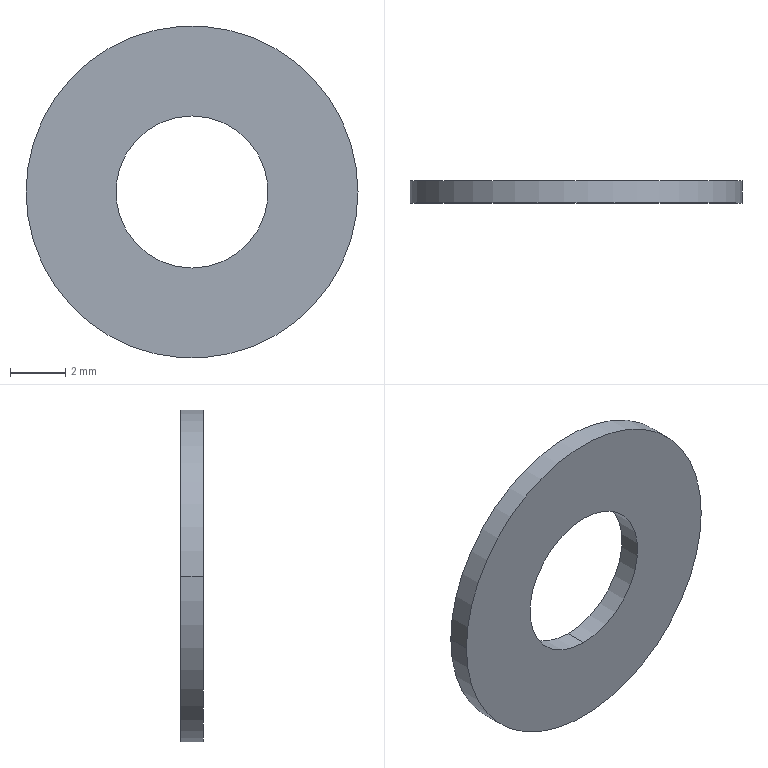Part | STEP file | ZZ21-M5 | 1 solid | 6 faces | box 12 x 0.8 x 12 mm | volume 71.471 mm3 | cylinder 4 | plane 2 | commonest cylinder face diameters 5.5 x2 12 x2
STEP:
#1=CARTESIAN_POINT('',(0.,0.,0.));
#2=DIRECTION('',(0.,0.,1.));
#3=DIRECTION('',(1.,0.,0.));
#4=AXIS2_PLACEMENT_3D('',#1,#2,#3);
#5=CARTESIAN_POINT('',(0.,0.,-2.75));
#6=VERTEX_POINT('',#5);
#7=CARTESIAN_POINT('',(0.,0.8,-2.75));
#8=VERTEX_POINT('',#7);
#9=CARTESIAN_POINT('',(0.,0.,-2.75));
#10=DIRECTION('',(0.,1.,0.));
#11=VECTOR('',#10,1.);
#12=LINE('',#9,#11);
#13=CARTESIAN_POINT('',(0.,0.,0.));
#14=DIRECTION('',(0.,1.,0.));
#15=DIRECTION('',(0.,0.,-1.));
#16=AXIS2_PLACEMENT_3D('',#13,#14,#15);
#17=CYLINDRICAL_SURFACE('',#16,2.75);
#18=CARTESIAN_POINT('',(6.283,0.));
#19=DIRECTION('',(0.,1.));
#20=VECTOR('',#19,1.);
#21=LINE('',#18,#20);
#22=(GEOMETRIC_REPRESENTATION_CONTEXT(2)PARAMETRIC_REPRESENTATION_CONTEXT()REPRESENTATION_CONTEXT('',''));
#23=DEFINITIONAL_REPRESENTATION('',(#21),#22);
#24=PCURVE('',#17,#23);
#25=CARTESIAN_POINT('',(0.,0.,0.));
#26=DIRECTION('',(0.,1.,0.));
#27=DIRECTION('',(0.,0.,-1.));
#28=AXIS2_PLACEMENT_3D('',#25,#26,#27);
#29=CYLINDRICAL_SURFACE('',#28,2.75);
#30=CARTESIAN_POINT('',(0.,0.));
#31=DIRECTION('',(0.,1.));
#32=VECTOR('',#31,1.);
#33=LINE('',#30,#32);
#34=(GEOMETRIC_REPRESENTATION_CONTEXT(2)PARAMETRIC_REPRESENTATION_CONTEXT()REPRESENTATION_CONTEXT('',''));
#35=DEFINITIONAL_REPRESENTATION('',(#33),#34);
#36=PCURVE('',#29,#35);
#37=SURFACE_CURVE('',#12,(#24,#36),.PCURVE_S1.);
#38=EDGE_CURVE('',#6,#8,#37,.T.);
#39=ORIENTED_EDGE('',*,*,#38,.T.);
#40=CARTESIAN_POINT('',(0.,0.8,2.75));
#41=VERTEX_POINT('',#40);
#42=CARTESIAN_POINT('',(0.,0.8,0.));
#43=DIRECTION('',(0.,-1.,0.));
#44=DIRECTION('',(0.,0.,1.));
#45=AXIS2_PLACEMENT_3D('',#42,#43,#44);
#46=CIRCLE('',#45,2.75);
#47=CARTESIAN_POINT('',(9.425,0.8));
#48=DIRECTION('',(-1.,0.));
#49=VECTOR('',#48,1.);
#50=LINE('',#47,#49);
#51=(GEOMETRIC_REPRESENTATION_CONTEXT(2)PARAMETRIC_REPRESENTATION_CONTEXT()REPRESENTATION_CONTEXT('',''));
#52=DEFINITIONAL_REPRESENTATION('',(#50),#51);
#53=PCURVE('',#17,#52);
#54=CARTESIAN_POINT('',(0.,0.8,0.));
#55=DIRECTION('',(0.,1.,0.));
#56=DIRECTION('',(-1.,0.,0.));
#57=AXIS2_PLACEMENT_3D('',#54,#55,#56);
#58=PLANE('',#57);
#59=CARTESIAN_POINT('',(0.,2.75));
#60=CARTESIAN_POINT('',(4.763,2.75));
#61=CARTESIAN_POINT('',(2.382,-1.375));
#62=CARTESIAN_POINT('',(0.,-5.5));
#63=CARTESIAN_POINT('',(-2.382,-1.375));
#64=CARTESIAN_POINT('',(-4.763,2.75));
#65=CARTESIAN_POINT('',(0.,2.75));
#66=(BOUNDED_CURVE()B_SPLINE_CURVE(2,(#59,#60,#61,#62,#63,#64,#65),.UNSPECIFIED.,.T.,.F.)B_SPLINE_CURVE_WITH_KNOTS((1,2,2,2,2,1),(-2.094,0.,2.094,4.189,6.283,8.378),.UNSPECIFIED.)CURVE()GEOMETRIC_REPRESENTATION_ITEM()RATIONAL_B_SPLINE_CURVE((1.,0.5,1.,0.5,1.,0.5,1.))REPRESENTATION_ITEM(''));
#67=(GEOMETRIC_REPRESENTATION_CONTEXT(2)PARAMETRIC_REPRESENTATION_CONTEXT()REPRESENTATION_CONTEXT('',''));
#68=DEFINITIONAL_REPRESENTATION('',(#66),#67);
#69=PCURVE('',#58,#68);
#70=SURFACE_CURVE('',#46,(#53,#69),.PCURVE_S1.);
#71=EDGE_CURVE('',#8,#41,#70,.T.);
#72=ORIENTED_EDGE('',*,*,#71,.T.);
#73=CARTESIAN_POINT('',(0.,0.,2.75));
#74=VERTEX_POINT('',#73);
#75=CARTESIAN_POINT('',(0.,0.,2.75));
#76=DIRECTION('',(0.,1.,0.));
#77=VECTOR('',#76,1.);
#78=LINE('',#75,#77);
#79=CARTESIAN_POINT('',(3.142,0.));
#80=DIRECTION('',(0.,1.));
#81=VECTOR('',#80,1.);
#82=LINE('',#79,#81);
#83=(GEOMETRIC_REPRESENTATION_CONTEXT(2)PARAMETRIC_REPRESENTATION_CONTEXT()REPRESENTATION_CONTEXT('',''));
#84=DEFINITIONAL_REPRESENTATION('',(#82),#83);
#85=PCURVE('',#17,#84);
#86=CARTESIAN_POINT('',(3.142,0.));
#87=DIRECTION('',(0.,1.));
#88=VECTOR('',#87,1.);
#89=LINE('',#86,#88);
#90=(GEOMETRIC_REPRESENTATION_CONTEXT(2)PARAMETRIC_REPRESENTATION_CONTEXT()REPRESENTATION_CONTEXT('',''));
#91=DEFINITIONAL_REPRESENTATION('',(#89),#90);
#92=PCURVE('',#29,#91);
#93=SURFACE_CURVE('',#78,(#85,#92),.PCURVE_S1.);
#94=EDGE_CURVE('',#74,#41,#93,.T.);
#95=ORIENTED_EDGE('',*,*,#94,.F.);
#96=CARTESIAN_POINT('',(0.,0.,0.));
#97=DIRECTION('',(0.,1.,0.));
#98=DIRECTION('',(0.,0.,-1.));
#99=AXIS2_PLACEMENT_3D('',#96,#97,#98);
#100=CIRCLE('',#99,2.75);
#101=CARTESIAN_POINT('',(0.,0.));
#102=DIRECTION('',(1.,0.));
#103=VECTOR('',#102,1.);
#104=LINE('',#101,#103);
#105=(GEOMETRIC_REPRESENTATION_CONTEXT(2)PARAMETRIC_REPRESENTATION_CONTEXT()REPRESENTATION_CONTEXT('',''));
#106=DEFINITIONAL_REPRESENTATION('',(#104),#105);
#107=PCURVE('',#17,#106);
#108=CARTESIAN_POINT('',(0.,0.,0.));
#109=DIRECTION('',(0.,-1.,0.));
#110=DIRECTION('',(1.,0.,0.));
#111=AXIS2_PLACEMENT_3D('',#108,#109,#110);
#112=PLANE('',#111);
#113=CARTESIAN_POINT('',(0.,-2.75));
#114=CARTESIAN_POINT('',(-4.763,-2.75));
#115=CARTESIAN_POINT('',(-2.382,1.375));
#116=CARTESIAN_POINT('',(0.,5.5));
#117=CARTESIAN_POINT('',(2.382,1.375));
#118=CARTESIAN_POINT('',(4.763,-2.75));
#119=CARTESIAN_POINT('',(0.,-2.75));
#120=(BOUNDED_CURVE()B_SPLINE_CURVE(2,(#113,#114,#115,#116,#117,#118,#119),.UNSPECIFIED.,.T.,.F.)B_SPLINE_CURVE_WITH_KNOTS((1,2,2,2,2,1),(-2.094,0.,2.094,4.189,6.283,8.378),.UNSPECIFIED.)CURVE()GEOMETRIC_REPRESENTATION_ITEM()RATIONAL_B_SPLINE_CURVE((1.,0.5,1.,0.5,1.,0.5,1.))REPRESENTATION_ITEM(''));
#121=(GEOMETRIC_REPRESENTATION_CONTEXT(2)PARAMETRIC_REPRESENTATION_CONTEXT()REPRESENTATION_CONTEXT('',''));
#122=DEFINITIONAL_REPRESENTATION('',(#120),#121);
#123=PCURVE('',#112,#122);
#124=SURFACE_CURVE('',#100,(#107,#123),.PCURVE_S1.);
#125=EDGE_CURVE('',#74,#6,#124,.T.);
#126=ORIENTED_EDGE('',*,*,#125,.T.);
#127=EDGE_LOOP('',(#39,#72,#95,#126));
#128=FACE_BOUND('',#127,.F.);
#129=ADVANCED_FACE('',(#128),#17,.F.);
#130=CARTESIAN_POINT('',(-6.,0.,0.));
#131=VERTEX_POINT('',#130);
#132=CARTESIAN_POINT('',(6.,0.,0.));
#133=VERTEX_POINT('',#132);
#134=CARTESIAN_POINT('',(0.,0.,0.));
#135=DIRECTION('',(0.,1.,0.));
#136=DIRECTION('',(-1.,0.,0.));
#137=AXIS2_PLACEMENT_3D('',#134,#135,#136);
#138=CIRCLE('',#137,6.);
#139=CARTESIAN_POINT('',(0.,0.,0.));
#140=DIRECTION('',(0.,1.,0.));
#141=DIRECTION('',(-1.,0.,0.));
#142=AXIS2_PLACEMENT_3D('',#139,#140,#141);
#143=CYLINDRICAL_SURFACE('',#142,6.);
#144=CARTESIAN_POINT('',(0.,0.));
#145=DIRECTION('',(1.,0.));
#146=VECTOR('',#145,1.);
#147=LINE('',#144,#146);
#148=(GEOMETRIC_REPRESENTATION_CONTEXT(2)PARAMETRIC_REPRESENTATION_CONTEXT()REPRESENTATION_CONTEXT('',''));
#149=DEFINITIONAL_REPRESENTATION('',(#147),#148);
#150=PCURVE('',#143,#149);
#151=CARTESIAN_POINT('',(-6.,0.));
#152=CARTESIAN_POINT('',(-6.,10.392));
#153=CARTESIAN_POINT('',(3.,5.196));
#154=CARTESIAN_POINT('',(12.,0.));
#155=CARTESIAN_POINT('',(3.,-5.196));
#156=CARTESIAN_POINT('',(-6.,-10.392));
#157=CARTESIAN_POINT('',(-6.,0.));
#158=(BOUNDED_CURVE()B_SPLINE_CURVE(2,(#151,#152,#153,#154,#155,#156,#157),.UNSPECIFIED.,.T.,.F.)B_SPLINE_CURVE_WITH_KNOTS((1,2,2,2,2,1),(-2.094,0.,2.094,4.189,6.283,8.378),.UNSPECIFIED.)CURVE()GEOMETRIC_REPRESENTATION_ITEM()RATIONAL_B_SPLINE_CURVE((1.,0.5,1.,0.5,1.,0.5,1.))REPRESENTATION_ITEM(''));
#159=(GEOMETRIC_REPRESENTATION_CONTEXT(2)PARAMETRIC_REPRESENTATION_CONTEXT()REPRESENTATION_CONTEXT('',''));
#160=DEFINITIONAL_REPRESENTATION('',(#158),#159);
#161=PCURVE('',#112,#160);
#162=SURFACE_CURVE('',#138,(#150,#161),.PCURVE_S1.);
#163=EDGE_CURVE('',#131,#133,#162,.T.);
#164=ORIENTED_EDGE('',*,*,#163,.T.);
#165=CARTESIAN_POINT('',(6.,0.8,0.));
#166=VERTEX_POINT('',#165);
#167=CARTESIAN_POINT('',(6.,0.,0.));
#168=DIRECTION('',(0.,1.,0.));
#169=VECTOR('',#168,1.);
#170=LINE('',#167,#169);
#171=CARTESIAN_POINT('',(3.142,0.));
#172=DIRECTION('',(0.,1.));
#173=VECTOR('',#172,1.);
#174=LINE('',#171,#173);
#175=(GEOMETRIC_REPRESENTATION_CONTEXT(2)PARAMETRIC_REPRESENTATION_CONTEXT()REPRESENTATION_CONTEXT('',''));
#176=DEFINITIONAL_REPRESENTATION('',(#174),#175);
#177=PCURVE('',#143,#176);
#178=CARTESIAN_POINT('',(0.,0.,0.));
#179=DIRECTION('',(0.,1.,0.));
#180=DIRECTION('',(-1.,0.,0.));
#181=AXIS2_PLACEMENT_3D('',#178,#179,#180);
#182=CYLINDRICAL_SURFACE('',#181,6.);
#183=CARTESIAN_POINT('',(3.142,0.));
#184=DIRECTION('',(0.,1.));
#185=VECTOR('',#184,1.);
#186=LINE('',#183,#185);
#187=(GEOMETRIC_REPRESENTATION_CONTEXT(2)PARAMETRIC_REPRESENTATION_CONTEXT()REPRESENTATION_CONTEXT('',''));
#188=DEFINITIONAL_REPRESENTATION('',(#186),#187);
#189=PCURVE('',#182,#188);
#190=SURFACE_CURVE('',#170,(#177,#189),.PCURVE_S1.);
#191=EDGE_CURVE('',#133,#166,#190,.T.);
#192=ORIENTED_EDGE('',*,*,#191,.T.);
#193=CARTESIAN_POINT('',(-6.,0.8,0.));
#194=VERTEX_POINT('',#193);
#195=CARTESIAN_POINT('',(0.,0.8,0.));
#196=DIRECTION('',(0.,-1.,0.));
#197=DIRECTION('',(1.,0.,0.));
#198=AXIS2_PLACEMENT_3D('',#195,#196,#197);
#199=CIRCLE('',#198,6.);
#200=CARTESIAN_POINT('',(3.142,0.8));
#201=DIRECTION('',(-1.,0.));
#202=VECTOR('',#201,1.);
#203=LINE('',#200,#202);
#204=(GEOMETRIC_REPRESENTATION_CONTEXT(2)PARAMETRIC_REPRESENTATION_CONTEXT()REPRESENTATION_CONTEXT('',''));
#205=DEFINITIONAL_REPRESENTATION('',(#203),#204);
#206=PCURVE('',#143,#205);
#207=CARTESIAN_POINT('',(-6.,0.));
#208=CARTESIAN_POINT('',(-6.,10.392));
#209=CARTESIAN_POINT('',(3.,5.196));
#210=CARTESIAN_POINT('',(12.,0.));
#211=CARTESIAN_POINT('',(3.,-5.196));
#212=CARTESIAN_POINT('',(-6.,-10.392));
#213=CARTESIAN_POINT('',(-6.,0.));
#214=(BOUNDED_CURVE()B_SPLINE_CURVE(2,(#207,#208,#209,#210,#211,#212,#213),.UNSPECIFIED.,.T.,.F.)B_SPLINE_CURVE_WITH_KNOTS((1,2,2,2,2,1),(-2.094,0.,2.094,4.189,6.283,8.378),.UNSPECIFIED.)CURVE()GEOMETRIC_REPRESENTATION_ITEM()RATIONAL_B_SPLINE_CURVE((1.,0.5,1.,0.5,1.,0.5,1.))REPRESENTATION_ITEM(''));
#215=(GEOMETRIC_REPRESENTATION_CONTEXT(2)PARAMETRIC_REPRESENTATION_CONTEXT()REPRESENTATION_CONTEXT('',''));
#216=DEFINITIONAL_REPRESENTATION('',(#214),#215);
#217=PCURVE('',#58,#216);
#218=SURFACE_CURVE('',#199,(#206,#217),.PCURVE_S1.);
#219=EDGE_CURVE('',#166,#194,#218,.T.);
#220=ORIENTED_EDGE('',*,*,#219,.T.);
#221=CARTESIAN_POINT('',(-6.,0.,0.));
#222=DIRECTION('',(0.,1.,0.));
#223=VECTOR('',#222,1.);
#224=LINE('',#221,#223);
#225=CARTESIAN_POINT('',(0.,0.));
#226=DIRECTION('',(0.,1.));
#227=VECTOR('',#226,1.);
#228=LINE('',#225,#227);
#229=(GEOMETRIC_REPRESENTATION_CONTEXT(2)PARAMETRIC_REPRESENTATION_CONTEXT()REPRESENTATION_CONTEXT('',''));
#230=DEFINITIONAL_REPRESENTATION('',(#228),#229);
#231=PCURVE('',#143,#230);
#232=CARTESIAN_POINT('',(6.283,0.));
#233=DIRECTION('',(0.,1.));
#234=VECTOR('',#233,1.);
#235=LINE('',#232,#234);
#236=(GEOMETRIC_REPRESENTATION_CONTEXT(2)PARAMETRIC_REPRESENTATION_CONTEXT()REPRESENTATION_CONTEXT('',''));
#237=DEFINITIONAL_REPRESENTATION('',(#235),#236);
#238=PCURVE('',#182,#237);
#239=SURFACE_CURVE('',#224,(#231,#238),.PCURVE_S1.);
#240=EDGE_CURVE('',#131,#194,#239,.T.);
#241=ORIENTED_EDGE('',*,*,#240,.F.);
#242=EDGE_LOOP('',(#164,#192,#220,#241));
#243=FACE_BOUND('',#242,.T.);
#244=ADVANCED_FACE('',(#243),#143,.T.);
#245=ORIENTED_EDGE('',*,*,#71,.T.);
#246=CARTESIAN_POINT('',(0.,0.8,0.));
#247=DIRECTION('',(0.,-1.,0.));
#248=DIRECTION('',(0.,0.,1.));
#249=AXIS2_PLACEMENT_3D('',#246,#247,#248);
#250=CIRCLE('',#249,2.75);
#251=CARTESIAN_POINT('',(0.,2.75));
#252=CARTESIAN_POINT('',(4.763,2.75));
#253=CARTESIAN_POINT('',(2.382,-1.375));
#254=CARTESIAN_POINT('',(0.,-5.5));
#255=CARTESIAN_POINT('',(-2.382,-1.375));
#256=CARTESIAN_POINT('',(-4.763,2.75));
#257=CARTESIAN_POINT('',(0.,2.75));
#258=(BOUNDED_CURVE()B_SPLINE_CURVE(2,(#251,#252,#253,#254,#255,#256,#257),.UNSPECIFIED.,.T.,.F.)B_SPLINE_CURVE_WITH_KNOTS((1,2,2,2,2,1),(-2.094,0.,2.094,4.189,6.283,8.378),.UNSPECIFIED.)CURVE()GEOMETRIC_REPRESENTATION_ITEM()RATIONAL_B_SPLINE_CURVE((1.,0.5,1.,0.5,1.,0.5,1.))REPRESENTATION_ITEM(''));
#259=(GEOMETRIC_REPRESENTATION_CONTEXT(2)PARAMETRIC_REPRESENTATION_CONTEXT()REPRESENTATION_CONTEXT('',''));
#260=DEFINITIONAL_REPRESENTATION('',(#258),#259);
#261=PCURVE('',#58,#260);
#262=CARTESIAN_POINT('',(3.142,0.8));
#263=DIRECTION('',(-1.,0.));
#264=VECTOR('',#263,1.);
#265=LINE('',#262,#264);
#266=(GEOMETRIC_REPRESENTATION_CONTEXT(2)PARAMETRIC_REPRESENTATION_CONTEXT()REPRESENTATION_CONTEXT('',''));
#267=DEFINITIONAL_REPRESENTATION('',(#265),#266);
#268=PCURVE('',#29,#267);
#269=SURFACE_CURVE('',#250,(#261,#268),.PCURVE_S1.);
#270=EDGE_CURVE('',#41,#8,#269,.T.);
#271=ORIENTED_EDGE('',*,*,#270,.T.);
#272=EDGE_LOOP('',(#245,#271));
#273=FACE_BOUND('',#272,.T.);
#274=CARTESIAN_POINT('',(0.,0.8,0.));
#275=DIRECTION('',(0.,-1.,0.));
#276=DIRECTION('',(1.,0.,0.));
#277=AXIS2_PLACEMENT_3D('',#274,#275,#276);
#278=CIRCLE('',#277,6.);
#279=CARTESIAN_POINT('',(-6.,0.));
#280=CARTESIAN_POINT('',(-6.,10.392));
#281=CARTESIAN_POINT('',(3.,5.196));
#282=CARTESIAN_POINT('',(12.,0.));
#283=CARTESIAN_POINT('',(3.,-5.196));
#284=CARTESIAN_POINT('',(-6.,-10.392));
#285=CARTESIAN_POINT('',(-6.,0.));
#286=(BOUNDED_CURVE()B_SPLINE_CURVE(2,(#279,#280,#281,#282,#283,#284,#285),.UNSPECIFIED.,.T.,.F.)B_SPLINE_CURVE_WITH_KNOTS((1,2,2,2,2,1),(-2.094,0.,2.094,4.189,6.283,8.378),.UNSPECIFIED.)CURVE()GEOMETRIC_REPRESENTATION_ITEM()RATIONAL_B_SPLINE_CURVE((1.,0.5,1.,0.5,1.,0.5,1.))REPRESENTATION_ITEM(''));
#287=(GEOMETRIC_REPRESENTATION_CONTEXT(2)PARAMETRIC_REPRESENTATION_CONTEXT()REPRESENTATION_CONTEXT('',''));
#288=DEFINITIONAL_REPRESENTATION('',(#286),#287);
#289=PCURVE('',#58,#288);
#290=CARTESIAN_POINT('',(9.425,0.8));
#291=DIRECTION('',(-1.,0.));
#292=VECTOR('',#291,1.);
#293=LINE('',#290,#292);
#294=(GEOMETRIC_REPRESENTATION_CONTEXT(2)PARAMETRIC_REPRESENTATION_CONTEXT()REPRESENTATION_CONTEXT('',''));
#295=DEFINITIONAL_REPRESENTATION('',(#293),#294);
#296=PCURVE('',#182,#295);
#297=SURFACE_CURVE('',#278,(#289,#296),.PCURVE_S1.);
#298=EDGE_CURVE('',#194,#166,#297,.T.);
#299=ORIENTED_EDGE('',*,*,#298,.F.);
#300=ORIENTED_EDGE('',*,*,#219,.F.);
#301=EDGE_LOOP('',(#299,#300));
#302=FACE_BOUND('',#301,.T.);
#303=ADVANCED_FACE('',(#273,#302),#58,.T.);
#304=CARTESIAN_POINT('',(0.,0.,0.));
#305=DIRECTION('',(0.,1.,0.));
#306=DIRECTION('',(0.,0.,-1.));
#307=AXIS2_PLACEMENT_3D('',#304,#305,#306);
#308=CIRCLE('',#307,2.75);
#309=CARTESIAN_POINT('',(0.,-2.75));
#310=CARTESIAN_POINT('',(-4.763,-2.75));
#311=CARTESIAN_POINT('',(-2.382,1.375));
#312=CARTESIAN_POINT('',(0.,5.5));
#313=CARTESIAN_POINT('',(2.382,1.375));
#314=CARTESIAN_POINT('',(4.763,-2.75));
#315=CARTESIAN_POINT('',(0.,-2.75));
#316=(BOUNDED_CURVE()B_SPLINE_CURVE(2,(#309,#310,#311,#312,#313,#314,#315),.UNSPECIFIED.,.T.,.F.)B_SPLINE_CURVE_WITH_KNOTS((1,2,2,2,2,1),(-2.094,0.,2.094,4.189,6.283,8.378),.UNSPECIFIED.)CURVE()GEOMETRIC_REPRESENTATION_ITEM()RATIONAL_B_SPLINE_CURVE((1.,0.5,1.,0.5,1.,0.5,1.))REPRESENTATION_ITEM(''));
#317=(GEOMETRIC_REPRESENTATION_CONTEXT(2)PARAMETRIC_REPRESENTATION_CONTEXT()REPRESENTATION_CONTEXT('',''));
#318=DEFINITIONAL_REPRESENTATION('',(#316),#317);
#319=PCURVE('',#112,#318);
#320=CARTESIAN_POINT('',(0.,0.));
#321=DIRECTION('',(1.,0.));
#322=VECTOR('',#321,1.);
#323=LINE('',#320,#322);
#324=(GEOMETRIC_REPRESENTATION_CONTEXT(2)PARAMETRIC_REPRESENTATION_CONTEXT()REPRESENTATION_CONTEXT('',''));
#325=DEFINITIONAL_REPRESENTATION('',(#323),#324);
#326=PCURVE('',#29,#325);
#327=SURFACE_CURVE('',#308,(#319,#326),.PCURVE_S1.);
#328=EDGE_CURVE('',#6,#74,#327,.T.);
#329=ORIENTED_EDGE('',*,*,#328,.T.);
#330=ORIENTED_EDGE('',*,*,#125,.T.);
#331=EDGE_LOOP('',(#329,#330));
#332=FACE_BOUND('',#331,.T.);
#333=ORIENTED_EDGE('',*,*,#163,.F.);
#334=CARTESIAN_POINT('',(0.,0.,0.));
#335=DIRECTION('',(0.,1.,0.));
#336=DIRECTION('',(-1.,0.,0.));
#337=AXIS2_PLACEMENT_3D('',#334,#335,#336);
#338=CIRCLE('',#337,6.);
#339=CARTESIAN_POINT('',(-6.,0.));
#340=CARTESIAN_POINT('',(-6.,10.392));
#341=CARTESIAN_POINT('',(3.,5.196));
#342=CARTESIAN_POINT('',(12.,0.));
#343=CARTESIAN_POINT('',(3.,-5.196));
#344=CARTESIAN_POINT('',(-6.,-10.392));
#345=CARTESIAN_POINT('',(-6.,0.));
#346=(BOUNDED_CURVE()B_SPLINE_CURVE(2,(#339,#340,#341,#342,#343,#344,#345),.UNSPECIFIED.,.T.,.F.)B_SPLINE_CURVE_WITH_KNOTS((1,2,2,2,2,1),(-2.094,0.,2.094,4.189,6.283,8.378),.UNSPECIFIED.)CURVE()GEOMETRIC_REPRESENTATION_ITEM()RATIONAL_B_SPLINE_CURVE((1.,0.5,1.,0.5,1.,0.5,1.))REPRESENTATION_ITEM(''));
#347=(GEOMETRIC_REPRESENTATION_CONTEXT(2)PARAMETRIC_REPRESENTATION_CONTEXT()REPRESENTATION_CONTEXT('',''));
#348=DEFINITIONAL_REPRESENTATION('',(#346),#347);
#349=PCURVE('',#112,#348);
#350=CARTESIAN_POINT('',(0.,0.));
#351=DIRECTION('',(1.,0.));
#352=VECTOR('',#351,1.);
#353=LINE('',#350,#352);
#354=(GEOMETRIC_REPRESENTATION_CONTEXT(2)PARAMETRIC_REPRESENTATION_CONTEXT()REPRESENTATION_CONTEXT('',''));
#355=DEFINITIONAL_REPRESENTATION('',(#353),#354);
#356=PCURVE('',#182,#355);
#357=SURFACE_CURVE('',#338,(#349,#356),.PCURVE_S1.);
#358=EDGE_CURVE('',#133,#131,#357,.T.);
#359=ORIENTED_EDGE('',*,*,#358,.F.);
#360=EDGE_LOOP('',(#333,#359));
#361=FACE_BOUND('',#360,.T.);
#362=ADVANCED_FACE('',(#332,#361),#112,.T.);
#363=ORIENTED_EDGE('',*,*,#191,.F.);
#364=ORIENTED_EDGE('',*,*,#358,.T.);
#365=ORIENTED_EDGE('',*,*,#240,.T.);
#366=ORIENTED_EDGE('',*,*,#298,.T.);
#367=EDGE_LOOP('',(#363,#364,#365,#366));
#368=FACE_BOUND('',#367,.T.);
#369=ADVANCED_FACE('',(#368),#182,.T.);
#370=ORIENTED_EDGE('',*,*,#270,.T.);
#371=ORIENTED_EDGE('',*,*,#38,.F.);
#372=ORIENTED_EDGE('',*,*,#328,.T.);
#373=ORIENTED_EDGE('',*,*,#94,.T.);
#374=EDGE_LOOP('',(#370,#371,#372,#373));
#375=FACE_BOUND('',#374,.F.);
#376=ADVANCED_FACE('',(#375),#29,.F.);
#377=CLOSED_SHELL('',(#129,#244,#303,#362,#369,#376));
#378=MANIFOLD_SOLID_BREP('',#377);
#379=(LENGTH_UNIT()NAMED_UNIT(*)SI_UNIT(.MILLI.,.METRE.));
#380=UNCERTAINTY_MEASURE_WITH_UNIT(LENGTH_MEASURE(0.0000001),#379,'','');
#381=(NAMED_UNIT(*)PLANE_ANGLE_UNIT()SI_UNIT($,.RADIAN.));
#382=(NAMED_UNIT(*)SI_UNIT($,.STERADIAN.)SOLID_ANGLE_UNIT());
#383=(GEOMETRIC_REPRESENTATION_CONTEXT(3)GLOBAL_UNCERTAINTY_ASSIGNED_CONTEXT((#380))GLOBAL_UNIT_ASSIGNED_CONTEXT((#379,#381,#382))REPRESENTATION_CONTEXT('',''));
#384=ADVANCED_BREP_SHAPE_REPRESENTATION('',(#4,#378),#383);